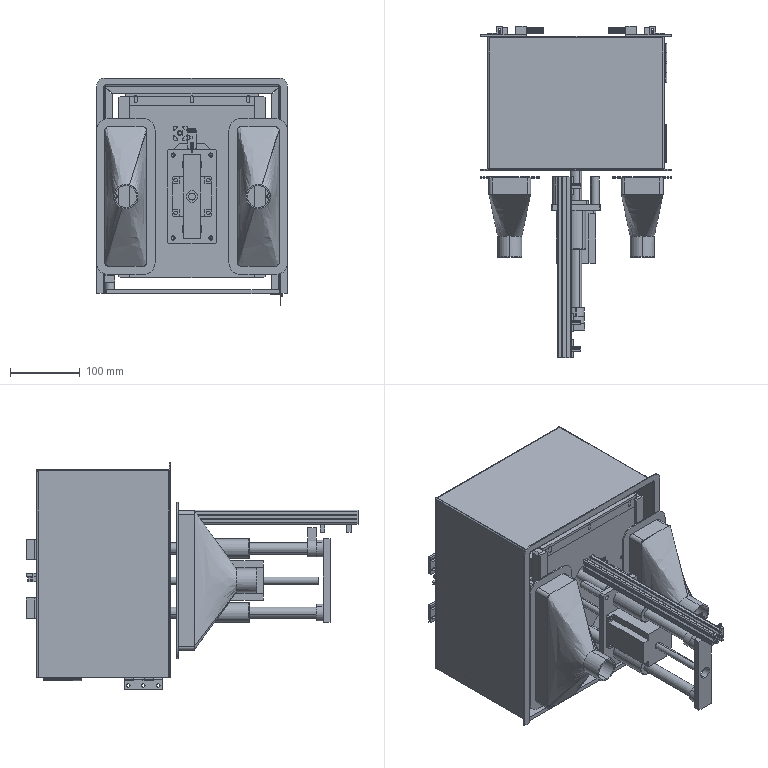Part | SolidWorks | 64 solids | 2014 faces | box 274 x 476.237 x 327 mm | volume 5964747 mm3 | plane 1135 | cylinder 775 | cone 88 | spline 16 | commonest cylinder face diameters 1 x280 5 x109 3.3 x52 4 x40 2.4 x24 3.2 x18